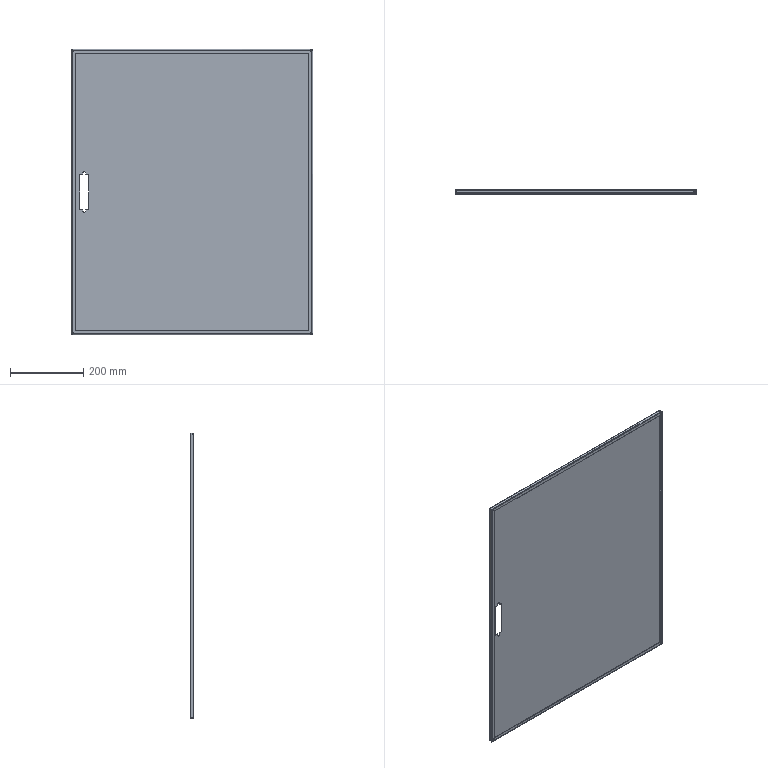Part | SolidWorks | features SMWeldBead 4, EdgeFlange 2, FlatPattern 1, HoleWzd 1, ICE 1, SMBaseFlange 1, SheetMetal 1 | 1 solid | 132 faces | box 659 x 10.5 x 779 mm | volume 836638 mm3 | plane 64 | spline 40 | cylinder 28 | commonest cylinder face diameters 1 x10 4 x8 2 x4 6 x4 7 x2